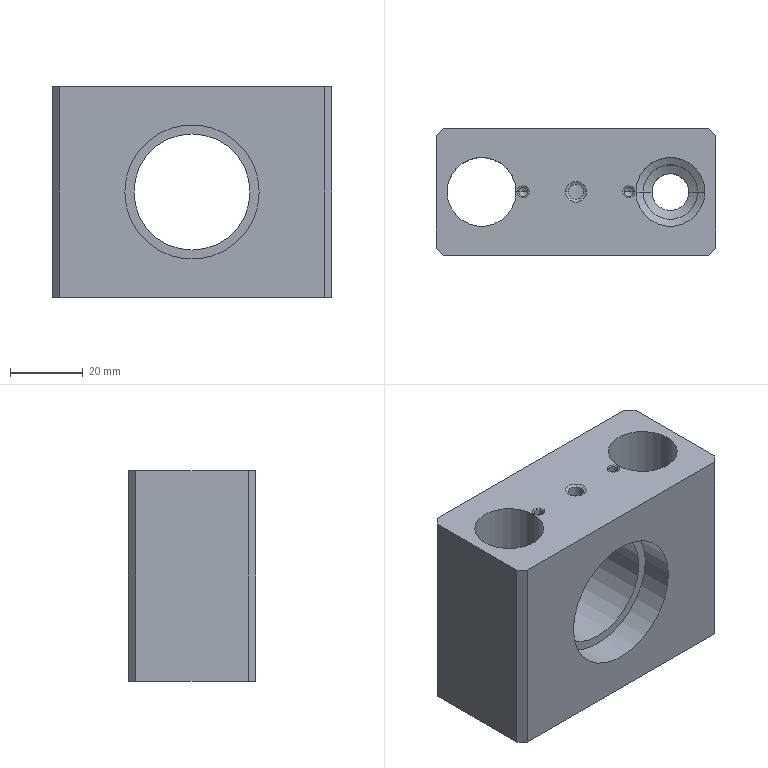Part | NX | 1 solid | 62 faces | box 77 x 35 x 58 mm | volume 93801 mm3 | cylinder 26 | cone 24 | plane 12 | commonest cylinder face diameters 2.5 x8 4.2 x4 19 x4 37 x4 10.1 x2 15 x2